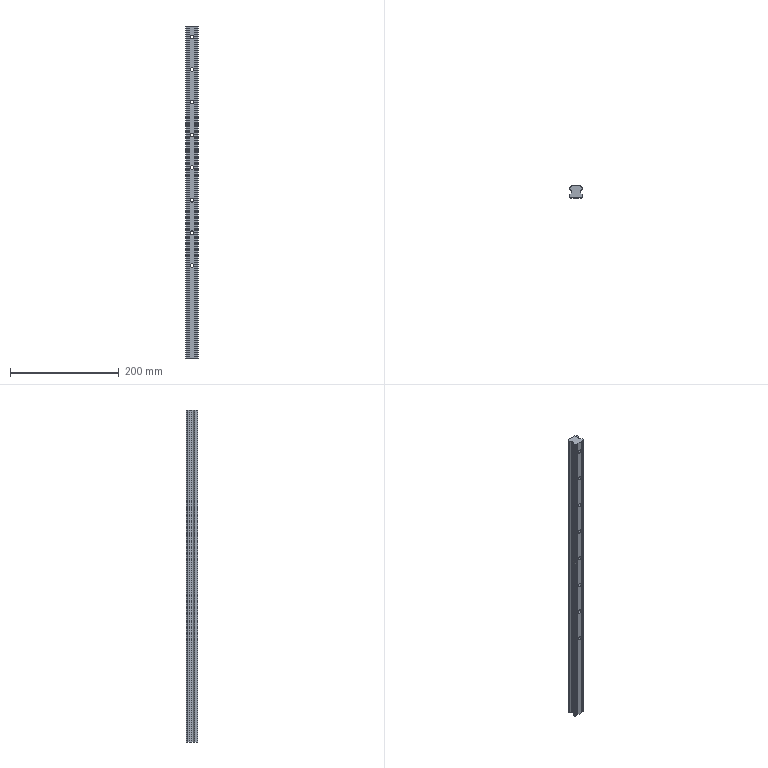Part | SolidWorks | features ICE 4, BaseBody 1, HoleWzd 1, LPattern 1 | 1 solid | 74 faces | box 23 x 22 x 610 mm | volume 258583 mm3 | plane 38 | cylinder 36 | commonest cylinder face diameters 11 x16 6.6 x10 7 x6 4.6 x4